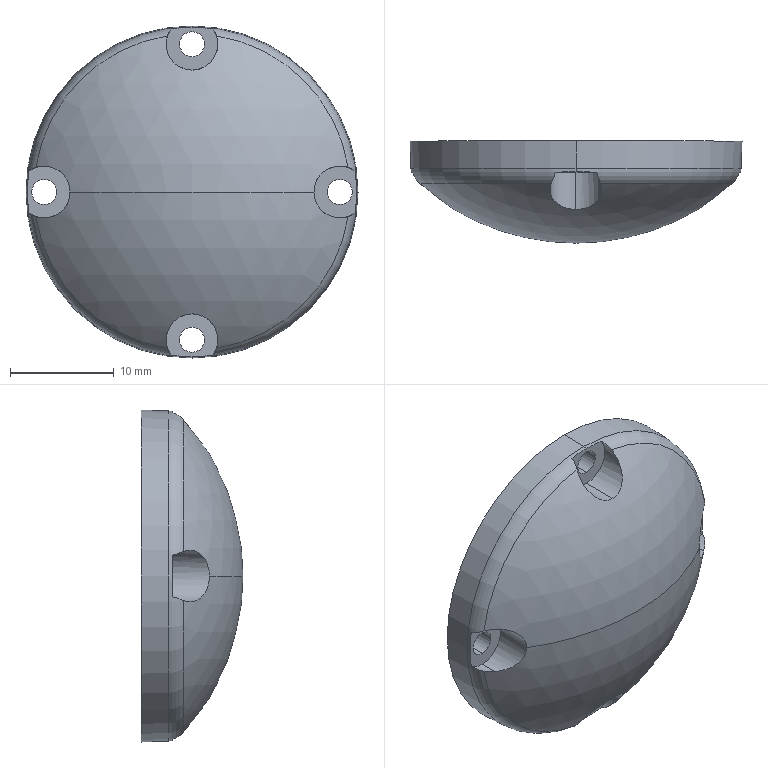Part | SolidWorks | features HoleWzd 1, Revolution 1 | 1 solid | 32 faces | box 32 x 9.828 x 32 mm | volume 4397 mm3 | cylinder 17 | plane 5 | sphere 4 | torus 4 | cone 2 | commonest cylinder face diameters 5 x9 2.4 x8
STEP:
#1=CARTESIAN_POINT('',(-14.25,-5.672,1.2));
#2=VERTEX_POINT('',#1);
#3=CARTESIAN_POINT('',(-14.25,-5.672,-1.2));
#4=VERTEX_POINT('',#3);
#5=CARTESIAN_POINT('',(-14.25,-5.672,0.));
#6=DIRECTION('',(0.,-1.,0.));
#7=DIRECTION('',(0.,0.,-1.));
#8=AXIS2_PLACEMENT_3D('',#5,#6,#7);
#9=CIRCLE('',#8,1.2);
#10=EDGE_CURVE('',#2,#4,#9,.T.);
#11=ORIENTED_EDGE('',*,*,#10,.F.);
#12=CARTESIAN_POINT('',(-14.25,-8.672,1.2));
#13=VERTEX_POINT('',#12);
#14=CARTESIAN_POINT('',(-14.25,-15.672,1.2));
#15=DIRECTION('',(0.,-1.,0.));
#16=VECTOR('',#15,1000.);
#17=LINE('',#14,#16);
#18=EDGE_CURVE('',#2,#13,#17,.T.);
#19=ORIENTED_EDGE('',*,*,#18,.T.);
#20=CARTESIAN_POINT('',(-14.25,-8.672,-1.2));
#21=VERTEX_POINT('',#20);
#22=CARTESIAN_POINT('',(-14.25,-8.672,0.));
#23=DIRECTION('',(0.,-1.,0.));
#24=DIRECTION('',(0.,0.,-1.));
#25=AXIS2_PLACEMENT_3D('',#22,#23,#24);
#26=CIRCLE('',#25,1.2);
#27=EDGE_CURVE('',#13,#21,#26,.T.);
#28=ORIENTED_EDGE('',*,*,#27,.T.);
#29=CARTESIAN_POINT('',(-14.25,-15.672,-1.2));
#30=DIRECTION('',(0.,-1.,0.));
#31=VECTOR('',#30,1000.);
#32=LINE('',#29,#31);
#33=EDGE_CURVE('',#4,#21,#32,.T.);
#34=ORIENTED_EDGE('',*,*,#33,.F.);
#35=EDGE_LOOP('',(#11,#19,#28,#34));
#36=FACE_OUTER_BOUND('',#35,.T.);
#37=CARTESIAN_POINT('',(-14.25,-15.672,0.));
#38=DIRECTION('',(0.,-1.,0.));
#39=DIRECTION('',(0.,0.,-1.));
#40=AXIS2_PLACEMENT_3D('',#37,#38,#39);
#41=CYLINDRICAL_SURFACE('',#40,1.2);
#42=ADVANCED_FACE('',(#36),#41,.F.);
#43=CARTESIAN_POINT('',(-14.25,-8.672,2.5));
#44=VERTEX_POINT('',#43);
#45=CARTESIAN_POINT('',(-15.732,-8.672,2.013));
#46=VERTEX_POINT('',#45);
#47=CARTESIAN_POINT('',(-14.25,-8.672,0.));
#48=DIRECTION('',(0.,-1.,0.));
#49=DIRECTION('',(0.,0.,-1.));
#50=AXIS2_PLACEMENT_3D('',#47,#48,#49);
#51=CIRCLE('',#50,2.5);
#52=EDGE_CURVE('',#44,#46,#51,.T.);
#53=ORIENTED_EDGE('',*,*,#52,.F.);
#54=CARTESIAN_POINT('',(-14.25,-10.38,2.5));
#55=VERTEX_POINT('',#54);
#56=CARTESIAN_POINT('',(-14.25,-15.672,2.5));
#57=DIRECTION('',(0.,-1.,0.));
#58=VECTOR('',#57,1000.);
#59=LINE('',#56,#58);
#60=EDGE_CURVE('',#44,#55,#59,.T.);
#61=ORIENTED_EDGE('',*,*,#60,.T.);
#62=CARTESIAN_POINT('',(-15.049,-9.731,2.369));
#63=VERTEX_POINT('',#62);
#64=CARTESIAN_POINT('',(-15.049,-9.731,2.369));
#65=CARTESIAN_POINT('',(-14.788,-9.947,2.457));
#66=CARTESIAN_POINT('',(-14.522,-10.163,2.5));
#67=CARTESIAN_POINT('',(-14.25,-10.38,2.5));
#68=B_SPLINE_CURVE_WITH_KNOTS('',3,(#64,#65,#66,#67),.UNSPECIFIED.,.F.,.F.,(4,4),(0.00000032,0.001037),.UNSPECIFIED.);
#69=EDGE_CURVE('',#63,#55,#68,.T.);
#70=ORIENTED_EDGE('',*,*,#69,.F.);
#71=CARTESIAN_POINT('',(-15.732,-8.672,2.013));
#72=CARTESIAN_POINT('',(-15.679,-8.886,2.053));
#73=CARTESIAN_POINT('',(-15.591,-9.079,2.114));
#74=CARTESIAN_POINT('',(-15.357,-9.436,2.245));
#75=CARTESIAN_POINT('',(-15.216,-9.594,2.313));
#76=CARTESIAN_POINT('',(-15.049,-9.731,2.369));
#77=B_SPLINE_CURVE_WITH_KNOTS('',3,(#71,#72,#73,#74,#75,#76),.UNSPECIFIED.,.F.,.F.,(4,2,4),(0.000000206,0.0006616,0.001323),.UNSPECIFIED.);
#78=EDGE_CURVE('',#46,#63,#77,.T.);
#79=ORIENTED_EDGE('',*,*,#78,.F.);
#80=EDGE_LOOP('',(#53,#61,#70,#79));
#81=FACE_OUTER_BOUND('',#80,.T.);
#82=CARTESIAN_POINT('',(-14.25,-15.672,0.));
#83=DIRECTION('',(0.,-1.,0.));
#84=DIRECTION('',(0.,0.,-1.));
#85=AXIS2_PLACEMENT_3D('',#82,#83,#84);
#86=CYLINDRICAL_SURFACE('',#85,2.5);
#87=ADVANCED_FACE('',(#81),#86,.F.);
#88=ORIENTED_EDGE('',*,*,#60,.F.);
#89=CARTESIAN_POINT('',(-14.25,-8.672,-2.5));
#90=VERTEX_POINT('',#89);
#91=CARTESIAN_POINT('',(-14.25,-8.672,0.));
#92=DIRECTION('',(0.,-1.,0.));
#93=DIRECTION('',(0.,0.,-1.));
#94=AXIS2_PLACEMENT_3D('',#91,#92,#93);
#95=CIRCLE('',#94,2.5);
#96=EDGE_CURVE('',#90,#44,#95,.T.);
#97=ORIENTED_EDGE('',*,*,#96,.F.);
#98=CARTESIAN_POINT('',(-14.25,-10.38,-2.5));
#99=VERTEX_POINT('',#98);
#100=CARTESIAN_POINT('',(-14.25,-15.672,-2.5));
#101=DIRECTION('',(0.,-1.,0.));
#102=VECTOR('',#101,1000.);
#103=LINE('',#100,#102);
#104=EDGE_CURVE('',#90,#99,#103,.T.);
#105=ORIENTED_EDGE('',*,*,#104,.T.);
#106=CARTESIAN_POINT('',(-11.75,-12.272,0.));
#107=VERTEX_POINT('',#106);
#108=CARTESIAN_POINT('',(-11.75,-12.272,0.));
#109=CARTESIAN_POINT('',(-11.75,-12.272,-0.1848));
#110=CARTESIAN_POINT('',(-11.77,-12.257,-0.3688));
#111=CARTESIAN_POINT('',(-11.851,-12.199,-0.7283));
#112=CARTESIAN_POINT('',(-11.91,-12.156,-0.8982));
#113=CARTESIAN_POINT('',(-12.136,-11.992,-1.381));
#114=CARTESIAN_POINT('',(-12.349,-11.836,-1.655));
#115=CARTESIAN_POINT('',(-12.833,-11.477,-2.085));
#116=CARTESIAN_POINT('',(-13.106,-11.271,-2.243));
#117=CARTESIAN_POINT('',(-13.668,-10.839,-2.45));
#118=CARTESIAN_POINT('',(-13.962,-10.609,-2.5));
#119=CARTESIAN_POINT('',(-14.25,-10.38,-2.5));
#120=B_SPLINE_CURVE_WITH_KNOTS('',3,(#108,#109,#110,#111,#112,#113,#114,#115,#116,#117,#118,#119),.UNSPECIFIED.,.F.,.F.,(4,2,2,2,2,4),(0.005459,0.00601,0.006561,0.007662,0.008764,0.009866),.UNSPECIFIED.);
#121=EDGE_CURVE('',#107,#99,#120,.T.);
#122=ORIENTED_EDGE('',*,*,#121,.F.);
#123=CARTESIAN_POINT('',(-14.25,-10.38,2.5));
#124=CARTESIAN_POINT('',(-14.105,-10.495,2.5));
#125=CARTESIAN_POINT('',(-13.958,-10.611,2.487));
#126=CARTESIAN_POINT('',(-13.671,-10.836,2.436));
#127=CARTESIAN_POINT('',(-13.529,-10.946,2.398));
#128=CARTESIAN_POINT('',(-13.109,-11.268,2.244));
#129=CARTESIAN_POINT('',(-12.834,-11.476,2.086));
#130=CARTESIAN_POINT('',(-12.472,-11.745,1.765));
#131=CARTESIAN_POINT('',(-12.357,-11.83,1.642));
#132=CARTESIAN_POINT('',(-12.152,-11.98,1.371));
#133=CARTESIAN_POINT('',(-12.062,-12.046,1.223));
#134=CARTESIAN_POINT('',(-11.911,-12.156,0.9004));
#135=CARTESIAN_POINT('',(-11.852,-12.199,0.7283));
#136=CARTESIAN_POINT('',(-11.771,-12.257,0.3733));
#137=CARTESIAN_POINT('',(-11.75,-12.272,0.1854));
#138=CARTESIAN_POINT('',(-11.75,-12.272,0.));
#139=B_SPLINE_CURVE_WITH_KNOTS('',3,(#123,#124,#125,#126,#127,#128,#129,#130,#131,#132,#133,#134,#135,#136,#137,#138),.UNSPECIFIED.,.F.,.F.,(4,2,2,2,2,2,2,4),(0.001037,0.00159,0.002142,0.003248,0.003801,0.004353,0.004906,0.005459),.UNSPECIFIED.);
#140=EDGE_CURVE('',#55,#107,#139,.T.);
#141=ORIENTED_EDGE('',*,*,#140,.F.);
#142=EDGE_LOOP('',(#88,#97,#105,#122,#141));
#143=FACE_OUTER_BOUND('',#142,.T.);
#144=CARTESIAN_POINT('',(-14.25,-15.672,0.));
#145=DIRECTION('',(0.,-1.,0.));
#146=DIRECTION('',(0.,0.,-1.));
#147=AXIS2_PLACEMENT_3D('',#144,#145,#146);
#148=CYLINDRICAL_SURFACE('',#147,2.5);
#149=ADVANCED_FACE('',(#143),#148,.F.);
#150=CARTESIAN_POINT('',(0.,-5.672,-13.05));
#151=VERTEX_POINT('',#150);
#152=CARTESIAN_POINT('',(0.,-5.672,-15.45));
#153=VERTEX_POINT('',#152);
#154=CARTESIAN_POINT('',(0.,-5.672,-14.25));
#155=DIRECTION('',(0.,-1.,0.));
#156=DIRECTION('',(0.,0.,-1.));
#157=AXIS2_PLACEMENT_3D('',#154,#155,#156);
#158=CIRCLE('',#157,1.2);
#159=EDGE_CURVE('',#151,#153,#158,.T.);
#160=ORIENTED_EDGE('',*,*,#159,.F.);
#161=CARTESIAN_POINT('',(0.,-8.672,-13.05));
#162=VERTEX_POINT('',#161);
#163=CARTESIAN_POINT('',(0.,-15.672,-13.05));
#164=DIRECTION('',(0.,-1.,0.));
#165=VECTOR('',#164,1000.);
#166=LINE('',#163,#165);
#167=EDGE_CURVE('',#151,#162,#166,.T.);
#168=ORIENTED_EDGE('',*,*,#167,.T.);
#169=CARTESIAN_POINT('',(0.,-8.672,-15.45));
#170=VERTEX_POINT('',#169);
#171=CARTESIAN_POINT('',(0.,-8.672,-14.25));
#172=DIRECTION('',(0.,-1.,0.));
#173=DIRECTION('',(0.,0.,-1.));
#174=AXIS2_PLACEMENT_3D('',#171,#172,#173);
#175=CIRCLE('',#174,1.2);
#176=EDGE_CURVE('',#162,#170,#175,.T.);
#177=ORIENTED_EDGE('',*,*,#176,.T.);
#178=CARTESIAN_POINT('',(0.,-15.672,-15.45));
#179=DIRECTION('',(0.,-1.,0.));
#180=VECTOR('',#179,1000.);
#181=LINE('',#178,#180);
#182=EDGE_CURVE('',#153,#170,#181,.T.);
#183=ORIENTED_EDGE('',*,*,#182,.F.);
#184=EDGE_LOOP('',(#160,#168,#177,#183));
#185=FACE_OUTER_BOUND('',#184,.T.);
#186=CARTESIAN_POINT('',(0.,-15.672,-14.25));
#187=DIRECTION('',(0.,-1.,0.));
#188=DIRECTION('',(0.,0.,-1.));
#189=AXIS2_PLACEMENT_3D('',#186,#187,#188);
#190=CYLINDRICAL_SURFACE('',#189,1.2);
#191=ADVANCED_FACE('',(#185),#190,.F.);
#192=CARTESIAN_POINT('',(14.25,-5.672,1.2));
#193=VERTEX_POINT('',#192);
#194=CARTESIAN_POINT('',(14.25,-5.672,-1.2));
#195=VERTEX_POINT('',#194);
#196=CARTESIAN_POINT('',(14.25,-5.672,0.));
#197=DIRECTION('',(0.,-1.,0.));
#198=DIRECTION('',(0.,0.,-1.));
#199=AXIS2_PLACEMENT_3D('',#196,#197,#198);
#200=CIRCLE('',#199,1.2);
#201=EDGE_CURVE('',#193,#195,#200,.T.);
#202=ORIENTED_EDGE('',*,*,#201,.F.);
#203=CARTESIAN_POINT('',(14.25,-8.672,1.2));
#204=VERTEX_POINT('',#203);
#205=CARTESIAN_POINT('',(14.25,-15.672,1.2));
#206=DIRECTION('',(0.,-1.,0.));
#207=VECTOR('',#206,1000.);
#208=LINE('',#205,#207);
#209=EDGE_CURVE('',#193,#204,#208,.T.);
#210=ORIENTED_EDGE('',*,*,#209,.T.);
#211=CARTESIAN_POINT('',(14.25,-8.672,-1.2));
#212=VERTEX_POINT('',#211);
#213=CARTESIAN_POINT('',(14.25,-8.672,0.));
#214=DIRECTION('',(0.,-1.,0.));
#215=DIRECTION('',(0.,0.,-1.));
#216=AXIS2_PLACEMENT_3D('',#213,#214,#215);
#217=CIRCLE('',#216,1.2);
#218=EDGE_CURVE('',#204,#212,#217,.T.);
#219=ORIENTED_EDGE('',*,*,#218,.T.);
#220=CARTESIAN_POINT('',(14.25,-15.672,-1.2));
#221=DIRECTION('',(0.,-1.,0.));
#222=VECTOR('',#221,1000.);
#223=LINE('',#220,#222);
#224=EDGE_CURVE('',#195,#212,#223,.T.);
#225=ORIENTED_EDGE('',*,*,#224,.F.);
#226=EDGE_LOOP('',(#202,#210,#219,#225));
#227=FACE_OUTER_BOUND('',#226,.T.);
#228=CARTESIAN_POINT('',(14.25,-15.672,0.));
#229=DIRECTION('',(0.,-1.,0.));
#230=DIRECTION('',(0.,0.,-1.));
#231=AXIS2_PLACEMENT_3D('',#228,#229,#230);
#232=CYLINDRICAL_SURFACE('',#231,1.2);
#233=ADVANCED_FACE('',(#227),#232,.F.);
#234=CARTESIAN_POINT('',(14.25,-8.672,2.5));
#235=VERTEX_POINT('',#234);
#236=CARTESIAN_POINT('',(14.25,-8.672,-2.5));
#237=VERTEX_POINT('',#236);
#238=CARTESIAN_POINT('',(14.25,-8.672,0.));
#239=DIRECTION('',(0.,-1.,0.));
#240=DIRECTION('',(0.,0.,-1.));
#241=AXIS2_PLACEMENT_3D('',#238,#239,#240);
#242=CIRCLE('',#241,2.5);
#243=EDGE_CURVE('',#235,#237,#242,.T.);
#244=ORIENTED_EDGE('',*,*,#243,.F.);
#245=CARTESIAN_POINT('',(14.25,-10.38,2.5));
#246=VERTEX_POINT('',#245);
#247=CARTESIAN_POINT('',(14.25,-15.672,2.5));
#248=DIRECTION('',(0.,-1.,0.));
#249=VECTOR('',#248,1000.);
#250=LINE('',#247,#249);
#251=EDGE_CURVE('',#235,#246,#250,.T.);
#252=ORIENTED_EDGE('',*,*,#251,.T.);
#253=CARTESIAN_POINT('',(11.75,-12.272,0.));
#254=VERTEX_POINT('',#253);
#255=CARTESIAN_POINT('',(11.75,-12.272,0.));
#256=CARTESIAN_POINT('',(11.75,-12.272,0.1848));
#257=CARTESIAN_POINT('',(11.77,-12.257,0.3688));
#258=CARTESIAN_POINT('',(11.851,-12.199,0.7283));
#259=CARTESIAN_POINT('',(11.91,-12.156,0.8982));
#260=CARTESIAN_POINT('',(12.136,-11.992,1.381));
#261=CARTESIAN_POINT('',(12.349,-11.836,1.655));
#262=CARTESIAN_POINT('',(12.833,-11.477,2.085));
#263=CARTESIAN_POINT('',(13.106,-11.271,2.243));
#264=CARTESIAN_POINT('',(13.668,-10.839,2.45));
#265=CARTESIAN_POINT('',(13.962,-10.609,2.5));
#266=CARTESIAN_POINT('',(14.25,-10.38,2.5));
#267=B_SPLINE_CURVE_WITH_KNOTS('',3,(#255,#256,#257,#258,#259,#260,#261,#262,#263,#264,#265,#266),.UNSPECIFIED.,.F.,.F.,(4,2,2,2,2,4),(0.005459,0.00601,0.006561,0.007662,0.008764,0.009866),.UNSPECIFIED.);
#268=EDGE_CURVE('',#254,#246,#267,.T.);
#269=ORIENTED_EDGE('',*,*,#268,.F.);
#270=CARTESIAN_POINT('',(14.25,-10.38,-2.5));
#271=VERTEX_POINT('',#270);
#272=CARTESIAN_POINT('',(14.25,-10.38,-2.5));
#273=CARTESIAN_POINT('',(14.105,-10.495,-2.5));
#274=CARTESIAN_POINT('',(13.958,-10.611,-2.487));
#275=CARTESIAN_POINT('',(13.671,-10.836,-2.436));
#276=CARTESIAN_POINT('',(13.529,-10.946,-2.398));
#277=CARTESIAN_POINT('',(13.109,-11.268,-2.244));
#278=CARTESIAN_POINT('',(12.834,-11.476,-2.086));
#279=CARTESIAN_POINT('',(12.472,-11.745,-1.765));
#280=CARTESIAN_POINT('',(12.357,-11.83,-1.642));
#281=CARTESIAN_POINT('',(12.152,-11.98,-1.371));
#282=CARTESIAN_POINT('',(12.062,-12.046,-1.223));
#283=CARTESIAN_POINT('',(11.911,-12.156,-0.9004));
#284=CARTESIAN_POINT('',(11.852,-12.199,-0.7283));
#285=CARTESIAN_POINT('',(11.771,-12.257,-0.3733));
#286=CARTESIAN_POINT('',(11.75,-12.272,-0.1854));
#287=CARTESIAN_POINT('',(11.75,-12.272,0.));
#288=B_SPLINE_CURVE_WITH_KNOTS('',3,(#272,#273,#274,#275,#276,#277,#278,#279,#280,#281,#282,#283,#284,#285,#286,#287),.UNSPECIFIED.,.F.,.F.,(4,2,2,2,2,2,2,4),(0.001037,0.00159,0.002142,0.003248,0.003801,0.004353,0.004906,0.005459),.UNSPECIFIED.);
#289=EDGE_CURVE('',#271,#254,#288,.T.);
#290=ORIENTED_EDGE('',*,*,#289,.F.);
#291=CARTESIAN_POINT('',(14.25,-15.672,-2.5));
#292=DIRECTION('',(0.,-1.,0.));
#293=VECTOR('',#292,1000.);
#294=LINE('',#291,#293);
#295=EDGE_CURVE('',#237,#271,#294,.T.);
#296=ORIENTED_EDGE('',*,*,#295,.F.);
#297=EDGE_LOOP('',(#244,#252,#269,#290,#296));
#298=FACE_OUTER_BOUND('',#297,.T.);
#299=CARTESIAN_POINT('',(14.25,-15.672,0.));
#300=DIRECTION('',(0.,-1.,0.));
#301=DIRECTION('',(0.,0.,-1.));
#302=AXIS2_PLACEMENT_3D('',#299,#300,#301);
#303=CYLINDRICAL_SURFACE('',#302,2.5);
#304=ADVANCED_FACE('',(#298),#303,.F.);
#305=CARTESIAN_POINT('',(15.732,-8.672,-2.013));
#306=VERTEX_POINT('',#305);
#307=CARTESIAN_POINT('',(14.25,-8.672,0.));
#308=DIRECTION('',(0.,-1.,0.));
#309=DIRECTION('',(0.,0.,-1.));
#310=AXIS2_PLACEMENT_3D('',#307,#308,#309);
#311=CIRCLE('',#310,2.5);
#312=EDGE_CURVE('',#237,#306,#311,.T.);
#313=ORIENTED_EDGE('',*,*,#312,.F.);
#314=ORIENTED_EDGE('',*,*,#295,.T.);
#315=CARTESIAN_POINT('',(15.049,-9.731,-2.369));
#316=VERTEX_POINT('',#315);
#317=CARTESIAN_POINT('',(15.049,-9.731,-2.369));
#318=CARTESIAN_POINT('',(14.788,-9.947,-2.457));
#319=CARTESIAN_POINT('',(14.522,-10.163,-2.5));
#320=CARTESIAN_POINT('',(14.25,-10.38,-2.5));
#321=B_SPLINE_CURVE_WITH_KNOTS('',3,(#317,#318,#319,#320),.UNSPECIFIED.,.F.,.F.,(4,4),(0.00000032,0.001037),.UNSPECIFIED.);
#322=EDGE_CURVE('',#316,#271,#321,.T.);
#323=ORIENTED_EDGE('',*,*,#322,.F.);
#324=CARTESIAN_POINT('',(15.732,-8.672,-2.013));
#325=CARTESIAN_POINT('',(15.679,-8.886,-2.053));
#326=CARTESIAN_POINT('',(15.591,-9.079,-2.114));
#327=CARTESIAN_POINT('',(15.357,-9.436,-2.245));
#328=CARTESIAN_POINT('',(15.216,-9.594,-2.313));
#329=CARTESIAN_POINT('',(15.049,-9.731,-2.369));
#330=B_SPLINE_CURVE_WITH_KNOTS('',3,(#324,#325,#326,#327,#328,#329),.UNSPECIFIED.,.F.,.F.,(4,2,4),(0.000000206,0.0006616,0.001323),.UNSPECIFIED.);
#331=EDGE_CURVE('',#306,#316,#330,.T.);
#332=ORIENTED_EDGE('',*,*,#331,.F.);
#333=EDGE_LOOP('',(#313,#314,#323,#332));
#334=FACE_OUTER_BOUND('',#333,.T.);
#335=CARTESIAN_POINT('',(14.25,-15.672,0.));
#336=DIRECTION('',(0.,-1.,0.));
#337=DIRECTION('',(0.,0.,-1.));
#338=AXIS2_PLACEMENT_3D('',#335,#336,#337);
#339=CYLINDRICAL_SURFACE('',#338,2.5);
#340=ADVANCED_FACE('',(#334),#339,.F.);
#341=CARTESIAN_POINT('',(0.,-5.672,15.45));
#342=VERTEX_POINT('',#341);
#343=CARTESIAN_POINT('',(0.,-5.672,13.05));
#344=VERTEX_POINT('',#343);
#345=CARTESIAN_POINT('',(0.,-5.672,14.25));
#346=DIRECTION('',(0.,-1.,0.));
#347=DIRECTION('',(0.,0.,-1.));
#348=AXIS2_PLACEMENT_3D('',#345,#346,#347);
#349=CIRCLE('',#348,1.2);
#350=EDGE_CURVE('',#342,#344,#349,.T.);
#351=ORIENTED_EDGE('',*,*,#350,.F.);
#352=CARTESIAN_POINT('',(0.,-8.672,15.45));
#353=VERTEX_POINT('',#352);
#354=CARTESIAN_POINT('',(0.,-15.672,15.45));
#355=DIRECTION('',(0.,-1.,0.));
#356=VECTOR('',#355,1000.);
#357=LINE('',#354,#356);
#358=EDGE_CURVE('',#342,#353,#357,.T.);
#359=ORIENTED_EDGE('',*,*,#358,.T.);
#360=CARTESIAN_POINT('',(0.,-8.672,13.05));
#361=VERTEX_POINT('',#360);
#362=CARTESIAN_POINT('',(0.,-8.672,14.25));
#363=DIRECTION('',(0.,-1.,0.));
#364=DIRECTION('',(0.,0.,-1.));
#365=AXIS2_PLACEMENT_3D('',#362,#363,#364);
#366=CIRCLE('',#365,1.2);
#367=EDGE_CURVE('',#353,#361,#366,.T.);
#368=ORIENTED_EDGE('',*,*,#367,.T.);
#369=CARTESIAN_POINT('',(0.,-15.672,13.05));
#370=DIRECTION('',(0.,-1.,0.));
#371=VECTOR('',#370,1000.);
#372=LINE('',#369,#371);
#373=EDGE_CURVE('',#344,#361,#372,.T.);
#374=ORIENTED_EDGE('',*,*,#373,.F.);
#375=EDGE_LOOP('',(#351,#359,#368,#374));
#376=FACE_OUTER_BOUND('',#375,.T.);
#377=CARTESIAN_POINT('',(0.,-15.672,14.25));
#378=DIRECTION('',(0.,-1.,0.));
#379=DIRECTION('',(0.,0.,-1.));
#380=AXIS2_PLACEMENT_3D('',#377,#378,#379);
#381=CYLINDRICAL_SURFACE('',#380,1.2);
#382=ADVANCED_FACE('',(#376),#381,.F.);
#383=CARTESIAN_POINT('',(0.,-8.672,11.75));
#384=VERTEX_POINT('',#383);
#385=CARTESIAN_POINT('',(2.013,-8.672,15.732));
#386=VERTEX_POINT('',#385);
#387=CARTESIAN_POINT('',(0.,-8.672,14.25));
#388=DIRECTION('',(0.,-1.,0.));
#389=DIRECTION('',(0.,0.,-1.));
#390=AXIS2_PLACEMENT_3D('',#387,#388,#389);
#391=CIRCLE('',#390,2.5);
#392=EDGE_CURVE('',#384,#386,#391,.T.);
#393=ORIENTED_EDGE('',*,*,#392,.F.);
#394=CARTESIAN_POINT('',(0.,-12.272,11.75));
#395=VERTEX_POINT('',#394);
#396=CARTESIAN_POINT('',(0.,-15.672,11.75));
#397=DIRECTION('',(0.,-1.,0.));
#398=VECTOR('',#397,1000.);
#399=LINE('',#396,#398);
#400=EDGE_CURVE('',#384,#395,#399,.T.);
#401=ORIENTED_EDGE('',*,*,#400,.T.);
#402=CARTESIAN_POINT('',(2.369,-9.731,15.049));
#403=VERTEX_POINT('',#402);
#404=CARTESIAN_POINT('',(2.369,-9.731,15.049));
#405=CARTESIAN_POINT('',(2.427,-9.873,14.877));
#406=CARTESIAN_POINT('',(2.465,-10.016,14.703));
#407=CARTESIAN_POINT('',(2.504,-10.3,14.35));
#408=CARTESIAN_POINT('',(2.505,-10.444,14.17));
#409=CARTESIAN_POINT('',(2.468,-10.727,13.811));
#410=CARTESIAN_POINT('',(2.43,-10.864,13.635));
#411=CARTESIAN_POINT('',(2.315,-11.132,13.288));
#412=CARTESIAN_POINT('',(2.236,-11.262,13.116));
#413=CARTESIAN_POINT('',(2.036,-11.511,12.786));
#414=CARTESIAN_POINT('',(1.915,-11.627,12.631));
#415=CARTESIAN_POINT('',(1.63,-11.84,12.343));
#416=CARTESIAN_POINT('',(1.463,-11.937,12.212));
#417=CARTESIAN_POINT('',(1.096,-12.096,11.993));
#418=CARTESIAN_POINT('',(0.8895,-12.162,11.903));
#419=CARTESIAN_POINT('',(0.5669,-12.227,11.813));
#420=CARTESIAN_POINT('',(0.4568,-12.244,11.789));
#421=CARTESIAN_POINT('',(0.2308,-12.266,11.758));
#422=CARTESIAN_POINT('',(0.1145,-12.272,11.75));
#423=CARTESIAN_POINT('',(0.,-12.272,11.75));
#424=B_SPLINE_CURVE_WITH_KNOTS('',3,(#404,#405,#406,#407,#408,#409,#410,#411,#412,#413,#414,#415,#416,#417,#418,#419,#420,#421,#422,#423),.UNSPECIFIED.,.F.,.F.,(4,2,2,2,2,2,2,2,2,4),(0.00000032,0.0006827,0.001365,0.002047,0.00273,0.003412,0.004094,0.004777,0.005118,0.005459),.UNSPECIFIED.);
#425=EDGE_CURVE('',#403,#395,#424,.T.);
#426=ORIENTED_EDGE('',*,*,#425,.F.);
#427=CARTESIAN_POINT('',(2.013,-8.672,15.732));
#428=CARTESIAN_POINT('',(2.053,-8.886,15.679));
#429=CARTESIAN_POINT('',(2.114,-9.079,15.591));
#430=CARTESIAN_POINT('',(2.245,-9.436,15.357));
#431=CARTESIAN_POINT('',(2.313,-9.594,15.216));
#432=CARTESIAN_POINT('',(2.369,-9.731,15.049));
#433=B_SPLINE_CURVE_WITH_KNOTS('',3,(#427,#428,#429,#430,#431,#432),.UNSPECIFIED.,.F.,.F.,(4,2,4),(0.000000206,0.0006616,0.001323),.UNSPECIFIED.);
#434=EDGE_CURVE('',#386,#403,#433,.T.);
#435=ORIENTED_EDGE('',*,*,#434,.F.);
#436=EDGE_LOOP('',(#393,#401,#426,#435));
#437=FACE_OUTER_BOUND('',#436,.T.);
#438=CARTESIAN_POINT('',(0.,-15.672,14.25));
#439=DIRECTION('',(0.,-1.,0.));
#440=DIRECTION('',(0.,0.,-1.));
#441=AXIS2_PLACEMENT_3D('',#438,#439,#440);
#442=CYLINDRICAL_SURFACE('',#441,2.5);
#443=ADVANCED_FACE('',(#437),#442,.F.);
#444=CARTESIAN_POINT('',(0.,-11.,0.));
#445=VERTEX_POINT('',#444);
#446=CARTESIAN_POINT('',(9.143,-6.116,0.));
#447=VERTEX_POINT('',#446);
#448=CARTESIAN_POINT('',(0.,0.,0.));
#449=DIRECTION('',(0.,0.,1.));
#450=DIRECTION('',(1.,0.,0.));
#451=AXIS2_PLACEMENT_3D('',#448,#449,#450);
#452=CIRCLE('',#451,11.);
#453=EDGE_CURVE('',#445,#447,#452,.T.);
#454=ORIENTED_EDGE('',*,*,#453,.F.);
#455=CARTESIAN_POINT('',(-9.143,-6.116,0.));
#456=VERTEX_POINT('',#455);
#457=CARTESIAN_POINT('',(0.,0.,0.));
#458=DIRECTION('',(0.,0.,-1.));
#459=DIRECTION('',(-1.,0.,0.));
#460=AXIS2_PLACEMENT_3D('',#457,#458,#459);
#461=CIRCLE('',#460,11.);
#462=EDGE_CURVE('',#445,#456,#461,.T.);
#463=ORIENTED_EDGE('',*,*,#462,.T.);
#464=CARTESIAN_POINT('',(0.,-6.116,9.143));
#465=VERTEX_POINT('',#464);
#466=CARTESIAN_POINT('',(0.,-6.116,0.));
#467=DIRECTION('',(0.,1.,0.));
#468=DIRECTION('',(0.,0.,1.));
#469=AXIS2_PLACEMENT_3D('',#466,#467,#468);
#470=CIRCLE('',#469,9.143);
#471=EDGE_CURVE('',#456,#465,#470,.T.);
#472=ORIENTED_EDGE('',*,*,#471,.T.);
#473=CARTESIAN_POINT('',(0.,-6.116,0.));
#474=DIRECTION('',(0.,1.,0.));
#475=DIRECTION('',(0.,0.,1.));
#476=AXIS2_PLACEMENT_3D('',#473,#474,#475);
#477=CIRCLE('',#476,9.143);
#478=EDGE_CURVE('',#465,#447,#477,.T.);
#479=ORIENTED_EDGE('',*,*,#478,.T.);
#480=EDGE_LOOP('',(#454,#463,#472,#479));
#481=FACE_OUTER_BOUND('',#480,.T.);
#482=CARTESIAN_POINT('',(0.,0.,0.));
#483=DIRECTION('',(0.,0.,-1.));
#484=DIRECTION('',(1.,0.,0.));
#485=AXIS2_PLACEMENT_3D('',#482,#483,#484);
#486=SPHERICAL_SURFACE('',#485,11.);
#487=ADVANCED_FACE('',(#481),#486,.F.);
#488=CARTESIAN_POINT('',(0.,-5.672,9.974));
#489=VERTEX_POINT('',#488);
#490=CARTESIAN_POINT('',(0.,-5.672,-9.974));
#491=VERTEX_POINT('',#490);
#492=CARTESIAN_POINT('',(0.,-5.672,0.));
#493=DIRECTION('',(0.,1.,0.));
#494=DIRECTION('',(0.,0.,1.));
#495=AXIS2_PLACEMENT_3D('',#492,#493,#494);
#496=CIRCLE('',#495,9.974);
#497=EDGE_CURVE('',#489,#491,#496,.T.);
#498=ORIENTED_EDGE('',*,*,#497,.T.);
#499=CARTESIAN_POINT('',(0.,-6.116,-9.143));
#500=VERTEX_POINT('',#499);
#501=CARTESIAN_POINT('',(0.,-6.672,-9.974));
#502=DIRECTION('',(1.,0.,0.));
#503=DIRECTION('',(0.,0.,-1.));
#504=AXIS2_PLACEMENT_3D('',#501,#502,#503);
#505=CIRCLE('',#504,1.);
#506=EDGE_CURVE('',#491,#500,#505,.T.);
#507=ORIENTED_EDGE('',*,*,#506,.T.);
#508=CARTESIAN_POINT('',(0.,-6.116,0.));
#509=DIRECTION('',(0.,1.,0.));
#510=DIRECTION('',(0.,0.,1.));
#511=AXIS2_PLACEMENT_3D('',#508,#509,#510);
#512=CIRCLE('',#511,9.143);
#513=EDGE_CURVE('',#447,#500,#512,.T.);
#514=ORIENTED_EDGE('',*,*,#513,.F.);
#515=ORIENTED_EDGE('',*,*,#478,.F.);
#516=CARTESIAN_POINT('',(0.,-6.672,9.974));
#517=DIRECTION('',(-1.,0.,0.));
#518=DIRECTION('',(0.,0.,1.));
#519=AXIS2_PLACEMENT_3D('',#516,#517,#518);
#520=CIRCLE('',#519,1.);
#521=EDGE_CURVE('',#489,#465,#520,.T.);
#522=ORIENTED_EDGE('',*,*,#521,.F.);
#523=EDGE_LOOP('',(#498,#507,#514,#515,#522));
#524=FACE_OUTER_BOUND('',#523,.T.);
#525=CARTESIAN_POINT('',(0.,-6.672,0.));
#526=DIRECTION('',(0.,1.,0.));
#527=DIRECTION('',(0.,0.,1.));
#528=AXIS2_PLACEMENT_3D('',#525,#526,#527);
#529=TOROIDAL_SURFACE('',#528,9.974,1.);
#530=ADVANCED_FACE('',(#524),#529,.T.);
#531=CARTESIAN_POINT('',(0.,-8.303,15.908));
#532=VERTEX_POINT('',#531);
#533=CARTESIAN_POINT('',(0.,-8.303,-15.908));
#534=VERTEX_POINT('',#533);
#535=CARTESIAN_POINT('',(0.,-8.303,0.));
#536=DIRECTION('',(0.,1.,0.));
#537=DIRECTION('',(0.,0.,1.));
#538=AXIS2_PLACEMENT_3D('',#535,#536,#537);
#539=CIRCLE('',#538,15.908);
#540=EDGE_CURVE('',#532,#534,#539,.T.);
#541=ORIENTED_EDGE('',*,*,#540,.T.);
#542=CARTESIAN_POINT('',(0.,-5.672,-16.));
#543=VERTEX_POINT('',#542);
#544=CARTESIAN_POINT('',(0.,-8.303,-15.908));
#545=DIRECTION('',(0.,0.9994,-0.0349));
#546=VECTOR('',#545,1000.);
#547=LINE('',#544,#546);
#548=EDGE_CURVE('',#534,#543,#547,.T.);
#549=ORIENTED_EDGE('',*,*,#548,.T.);
#550=CARTESIAN_POINT('',(0.,-5.672,16.));
#551=VERTEX_POINT('',#550);
#552=CARTESIAN_POINT('',(0.,-5.672,0.));
#553=DIRECTION('',(0.,1.,0.));
#554=DIRECTION('',(0.,0.,1.));
#555=AXIS2_PLACEMENT_3D('',#552,#553,#554);
#556=CIRCLE('',#555,16.);
#557=EDGE_CURVE('',#551,#543,#556,.T.);
#558=ORIENTED_EDGE('',*,*,#557,.F.);
#559=CARTESIAN_POINT('',(0.,-8.303,15.908));
#560=DIRECTION('',(0.,0.9994,0.0349));
#561=VECTOR('',#560,1000.);
#562=LINE('',#559,#561);
#563=EDGE_CURVE('',#532,#551,#562,.T.);
#564=ORIENTED_EDGE('',*,*,#563,.F.);
#565=EDGE_LOOP('',(#541,#549,#558,#564));
#566=FACE_OUTER_BOUND('',#565,.T.);
#567=CARTESIAN_POINT('',(0.,-8.303,0.));
#568=DIRECTION('',(0.,1.,0.));
#569=DIRECTION('',(0.,0.,1.));
#570=AXIS2_PLACEMENT_3D('',#567,#568,#569);
#571=CONICAL_SURFACE('',#570,15.908,0.03491);
#572=ADVANCED_FACE('',(#566),#571,.T.);
#573=CARTESIAN_POINT('',(2.013,-8.672,-15.732));
#574=VERTEX_POINT('',#573);
#575=CARTESIAN_POINT('',(0.,-8.672,-15.861));
#576=VERTEX_POINT('',#575);
#577=CARTESIAN_POINT('',(0.,-8.672,0.));
#578=DIRECTION('',(0.,1.,0.));
#579=DIRECTION('',(0.,0.,1.));
#580=AXIS2_PLACEMENT_3D('',#577,#578,#579);
#581=CIRCLE('',#580,15.861);
#582=EDGE_CURVE('',#574,#576,#581,.T.);
#583=ORIENTED_EDGE('',*,*,#582,.T.);
#584=CARTESIAN_POINT('',(0.,-8.233,-13.909));
#585=DIRECTION('',(1.,0.,0.));
#586=DIRECTION('',(0.,0.,-1.));
#587=AXIS2_PLACEMENT_3D('',#584,#585,#586);
#588=CIRCLE('',#587,2.);
#589=EDGE_CURVE('',#576,#534,#588,.T.);
#590=ORIENTED_EDGE('',*,*,#589,.T.);
#591=ORIENTED_EDGE('',*,*,#540,.F.);
#592=CARTESIAN_POINT('',(0.,-8.672,15.861));
#593=VERTEX_POINT('',#592);
#594=CARTESIAN_POINT('',(0.,-8.233,13.909));
#595=DIRECTION('',(-1.,0.,0.));
#596=DIRECTION('',(0.,0.,1.));
#597=AXIS2_PLACEMENT_3D('',#594,#595,#596);
#598=CIRCLE('',#597,2.);
#599=EDGE_CURVE('',#593,#532,#598,.T.);
#600=ORIENTED_EDGE('',*,*,#599,.F.);
#601=CARTESIAN_POINT('',(0.,-8.672,0.));
#602=DIRECTION('',(0.,1.,0.));
#603=DIRECTION('',(0.,0.,1.));
#604=AXIS2_PLACEMENT_3D('',#601,#602,#603);
#605=CIRCLE('',#604,15.861);
#606=EDGE_CURVE('',#593,#386,#605,.T.);
#607=ORIENTED_EDGE('',*,*,#606,.T.);
#608=ORIENTED_EDGE('',*,*,#434,.T.);
#609=CARTESIAN_POINT('',(15.049,-9.731,2.369));
#610=VERTEX_POINT('',#609);
#611=CARTESIAN_POINT('',(0.,-9.731,0.));
#612=DIRECTION('',(0.,1.,0.));
#613=DIRECTION('',(0.,0.,1.));
#614=AXIS2_PLACEMENT_3D('',#611,#612,#613);
#615=CIRCLE('',#614,15.234);
#616=EDGE_CURVE('',#403,#610,#615,.T.);
#617=ORIENTED_EDGE('',*,*,#616,.T.);
#618=CARTESIAN_POINT('',(15.732,-8.672,2.013));
#619=VERTEX_POINT('',#618);
#620=CARTESIAN_POINT('',(15.049,-9.731,2.369));
#621=CARTESIAN_POINT('',(15.216,-9.593,2.313));
#622=CARTESIAN_POINT('',(15.356,-9.437,2.246));
#623=CARTESIAN_POINT('',(15.59,-9.081,2.115));
#624=CARTESIAN_POINT('',(15.679,-8.886,2.053));
#625=CARTESIAN_POINT('',(15.732,-8.672,2.013));
#626=B_SPLINE_CURVE_WITH_KNOTS('',3,(#620,#621,#622,#623,#624,#625),.UNSPECIFIED.,.F.,.F.,(4,2,4),(0.00000032,0.0006625,0.001325),.UNSPECIFIED.);
#627=EDGE_CURVE('',#610,#619,#626,.T.);
#628=ORIENTED_EDGE('',*,*,#627,.T.);
#629=CARTESIAN_POINT('',(0.,-8.672,0.));
#630=DIRECTION('',(0.,1.,0.));
#631=DIRECTION('',(0.,0.,1.));
#632=AXIS2_PLACEMENT_3D('',#629,#630,#631);
#633=CIRCLE('',#632,15.861);
#634=EDGE_CURVE('',#619,#306,#633,.T.);
#635=ORIENTED_EDGE('',*,*,#634,.T.);
#636=ORIENTED_EDGE('',*,*,#331,.T.);
#637=CARTESIAN_POINT('',(2.369,-9.731,-15.049));
#638=VERTEX_POINT('',#637);
#639=CARTESIAN_POINT('',(0.,-9.731,0.));
#640=DIRECTION('',(0.,1.,0.));
#641=DIRECTION('',(0.,0.,1.));
#642=AXIS2_PLACEMENT_3D('',#639,#640,#641);
#643=CIRCLE('',#642,15.234);
#644=EDGE_CURVE('',#316,#638,#643,.T.);
#645=ORIENTED_EDGE('',*,*,#644,.T.);
#646=CARTESIAN_POINT('',(2.369,-9.731,-15.049));
#647=CARTESIAN_POINT('',(2.313,-9.593,-15.216));
#648=CARTESIAN_POINT('',(2.246,-9.437,-15.356));
#649=CARTESIAN_POINT('',(2.115,-9.081,-15.59));
#650=CARTESIAN_POINT('',(2.053,-8.886,-15.679));
#651=CARTESIAN_POINT('',(2.013,-8.672,-15.732));
#652=B_SPLINE_CURVE_WITH_KNOTS('',3,(#646,#647,#648,#649,#650,#651),.UNSPECIFIED.,.F.,.F.,(4,2,4),(0.00000032,0.0006625,0.001325),.UNSPECIFIED.);
#653=EDGE_CURVE('',#638,#574,#652,.T.);
#654=ORIENTED_EDGE('',*,*,#653,.T.);
#655=EDGE_LOOP('',(#583,#590,#591,#600,#607,#608,#617,#628,#635,#636,#645,#654));
#656=FACE_OUTER_BOUND('',#655,.T.);
#657=CARTESIAN_POINT('',(0.,-8.233,0.));
#658=DIRECTION('',(0.,1.,0.));
#659=DIRECTION('',(0.,0.,1.));
#660=AXIS2_PLACEMENT_3D('',#657,#658,#659);
#661=TOROIDAL_SURFACE('',#660,13.909,2.);
#662=ADVANCED_FACE('',(#656),#661,.T.);
#663=CARTESIAN_POINT('',(0.,-15.5,0.));
#664=VERTEX_POINT('',#663);
#665=CARTESIAN_POINT('',(0.,7.5,0.));
#666=DIRECTION('',(0.,0.,1.));
#667=DIRECTION('',(1.,0.,0.));
#668=AXIS2_PLACEMENT_3D('',#665,#666,#667);
#669=CIRCLE('',#668,23.);
#670=EDGE_CURVE('',#664,#254,#669,.T.);
#671=ORIENTED_EDGE('',*,*,#670,.F.);
#672=CARTESIAN_POINT('',(0.,7.5,0.));
#673=DIRECTION('',(0.,0.,-1.));
#674=DIRECTION('',(-1.,0.,0.));
#675=AXIS2_PLACEMENT_3D('',#672,#673,#674);
#676=CIRCLE('',#675,23.);
#677=EDGE_CURVE('',#664,#107,#676,.T.);
#678=ORIENTED_EDGE('',*,*,#677,.T.);
#679=ORIENTED_EDGE('',*,*,#121,.T.);
#680=CARTESIAN_POINT('',(-15.049,-9.731,-2.369));
#681=VERTEX_POINT('',#680);
#682=CARTESIAN_POINT('',(-14.25,-10.38,-2.5));
#683=CARTESIAN_POINT('',(-14.519,-10.165,-2.5));
#684=CARTESIAN_POINT('',(-14.789,-9.946,-2.457));
#685=CARTESIAN_POINT('',(-15.049,-9.731,-2.369));
#686=B_SPLINE_CURVE_WITH_KNOTS('',3,(#682,#683,#684,#685),.UNSPECIFIED.,.F.,.F.,(4,4),(0.009866,0.0109),.UNSPECIFIED.);
#687=EDGE_CURVE('',#99,#681,#686,.T.);
#688=ORIENTED_EDGE('',*,*,#687,.T.);
#689=CARTESIAN_POINT('',(-2.369,-9.731,-15.049));
#690=VERTEX_POINT('',#689);
#691=CARTESIAN_POINT('',(0.,-9.731,0.));
#692=DIRECTION('',(0.,1.,0.));
#693=DIRECTION('',(0.,0.,1.));
#694=AXIS2_PLACEMENT_3D('',#691,#692,#693);
#695=CIRCLE('',#694,15.234);
#696=EDGE_CURVE('',#690,#681,#695,.T.);
#697=ORIENTED_EDGE('',*,*,#696,.F.);
#698=CARTESIAN_POINT('',(-2.369,-9.731,-15.049));
#699=CARTESIAN_POINT('',(-2.427,-9.873,-14.877));
#700=CARTESIAN_POINT('',(-2.465,-10.015,-14.704));
#701=CARTESIAN_POINT('',(-2.504,-10.299,-14.352));
#702=CARTESIAN_POINT('',(-2.505,-10.442,-14.172));
#703=CARTESIAN_POINT('',(-2.468,-10.725,-13.814));
#704=CARTESIAN_POINT('',(-2.431,-10.862,-13.638));
#705=CARTESIAN_POINT('',(-2.316,-11.129,-13.291));
#706=CARTESIAN_POINT('',(-2.238,-11.26,-13.12));
#707=CARTESIAN_POINT('',(-2.038,-11.508,-12.79));
#708=CARTESIAN_POINT('',(-1.919,-11.624,-12.635));
#709=CARTESIAN_POINT('',(-1.635,-11.837,-12.348));
#710=CARTESIAN_POINT('',(-1.469,-11.934,-12.216));
#711=CARTESIAN_POINT('',(-1.104,-12.094,-11.997));
#712=CARTESIAN_POINT('',(-0.8978,-12.159,-11.906));
#713=CARTESIAN_POINT('',(-0.5764,-12.225,-11.815));
#714=CARTESIAN_POINT('',(-0.4666,-12.242,-11.791));
#715=CARTESIAN_POINT('',(-0.2414,-12.266,-11.759));
#716=CARTESIAN_POINT('',(-0.1253,-12.272,-11.751));
#717=CARTESIAN_POINT('',(0.1032,-12.272,-11.75));
#718=CARTESIAN_POINT('',(0.2168,-12.267,-11.757));
#719=CARTESIAN_POINT('',(0.4424,-12.246,-11.787));
#720=CARTESIAN_POINT('',(0.5553,-12.229,-11.81));
#721=CARTESIAN_POINT('',(0.8808,-12.164,-11.9));
#722=CARTESIAN_POINT('',(1.086,-12.1,-11.988));
#723=CARTESIAN_POINT('',(1.456,-11.941,-12.206));
#724=CARTESIAN_POINT('',(1.621,-11.845,-12.336));
#725=CARTESIAN_POINT('',(1.91,-11.632,-12.624));
#726=CARTESIAN_POINT('',(2.031,-11.516,-12.779));
#727=CARTESIAN_POINT('',(2.233,-11.268,-13.109));
#728=CARTESIAN_POINT('',(2.312,-11.137,-13.28));
#729=CARTESIAN_POINT('',(2.429,-10.868,-13.63));
#730=CARTESIAN_POINT('',(2.468,-10.727,-13.81));
#731=CARTESIAN_POINT('',(2.505,-10.446,-14.168));
#732=CARTESIAN_POINT('',(2.505,-10.304,-14.346));
#733=CARTESIAN_POINT('',(2.466,-10.018,-14.7));
#734=CARTESIAN_POINT('',(2.427,-9.873,-14.877));
#735=CARTESIAN_POINT('',(2.369,-9.731,-15.049));
#736=B_SPLINE_CURVE_WITH_KNOTS('',3,(#698,#699,#700,#701,#702,#703,#704,#705,#706,#707,#708,#709,#710,#711,#712,#713,#714,#715,#716,#717,#718,#719,#720,#721,#722,#723,#724,#725,#726,#727,#728,#729,#730,#731,#732,#733,#734,#735),.UNSPECIFIED.,.F.,.F.,(4,2,2,2,2,2,2,2,2,2,2,2,2,2,2,2,2,2,4),(0.00000032,0.0006813,0.001362,0.002043,0.002724,0.003405,0.004086,0.004767,0.005108,0.005448,0.005789,0.006129,0.00681,0.007491,0.008172,0.008853,0.009534,0.01021,0.0109),.UNSPECIFIED.);
#737=EDGE_CURVE('',#690,#638,#736,.T.);
#738=ORIENTED_EDGE('',*,*,#737,.T.);
#739=ORIENTED_EDGE('',*,*,#644,.F.);
#740=ORIENTED_EDGE('',*,*,#322,.T.);
#741=ORIENTED_EDGE('',*,*,#289,.T.);
#742=EDGE_LOOP('',(#671,#678,#679,#688,#697,#738,#739,#740,#741));
#743=FACE_OUTER_BOUND('',#742,.T.);
#744=CARTESIAN_POINT('',(0.,7.5,0.));
#745=DIRECTION('',(0.,0.,-1.));
#746=DIRECTION('',(1.,0.,0.));
#747=AXIS2_PLACEMENT_3D('',#744,#745,#746);
#748=SPHERICAL_SURFACE('',#747,23.);
#749=ADVANCED_FACE('',(#743),#748,.T.);
#750=ORIENTED_EDGE('',*,*,#677,.F.);
#751=ORIENTED_EDGE('',*,*,#670,.T.);
#752=ORIENTED_EDGE('',*,*,#268,.T.);
#753=CARTESIAN_POINT('',(14.25,-10.38,2.5));
#754=CARTESIAN_POINT('',(14.519,-10.165,2.5));
#755=CARTESIAN_POINT('',(14.789,-9.946,2.457));
#756=CARTESIAN_POINT('',(15.049,-9.731,2.369));
#757=B_SPLINE_CURVE_WITH_KNOTS('',3,(#753,#754,#755,#756),.UNSPECIFIED.,.F.,.F.,(4,4),(0.009866,0.0109),.UNSPECIFIED.);
#758=EDGE_CURVE('',#246,#610,#757,.T.);
#759=ORIENTED_EDGE('',*,*,#758,.T.);
#760=ORIENTED_EDGE('',*,*,#616,.F.);
#761=ORIENTED_EDGE('',*,*,#425,.T.);
#762=CARTESIAN_POINT('',(-2.369,-9.731,15.049));
#763=VERTEX_POINT('',#762);
#764=CARTESIAN_POINT('',(0.,-12.272,11.75));
#765=CARTESIAN_POINT('',(-0.114,-12.272,11.75));
#766=CARTESIAN_POINT('',(-0.2273,-12.267,11.758));
#767=CARTESIAN_POINT('',(-0.4524,-12.244,11.789));
#768=CARTESIAN_POINT('',(-0.5649,-12.227,11.812));
#769=CARTESIAN_POINT('',(-0.8891,-12.162,11.903));
#770=CARTESIAN_POINT('',(-1.093,-12.097,11.992));
#771=CARTESIAN_POINT('',(-1.462,-11.937,12.211));
#772=CARTESIAN_POINT('',(-1.627,-11.842,12.341));
#773=CARTESIAN_POINT('',(-1.913,-11.629,12.628));
#774=CARTESIAN_POINT('',(-2.034,-11.513,12.783));
#775=CARTESIAN_POINT('',(-2.235,-11.265,13.113));
#776=CARTESIAN_POINT('',(-2.313,-11.134,13.284));
#777=CARTESIAN_POINT('',(-2.43,-10.866,13.633));
#778=CARTESIAN_POINT('',(-2.468,-10.725,13.813));
#779=CARTESIAN_POINT('',(-2.505,-10.444,14.17));
#780=CARTESIAN_POINT('',(-2.504,-10.303,14.347));
#781=CARTESIAN_POINT('',(-2.465,-10.017,14.701));
#782=CARTESIAN_POINT('',(-2.427,-9.873,14.877));
#783=CARTESIAN_POINT('',(-2.369,-9.731,15.049));
#784=B_SPLINE_CURVE_WITH_KNOTS('',3,(#764,#765,#766,#767,#768,#769,#770,#771,#772,#773,#774,#775,#776,#777,#778,#779,#780,#781,#782,#783),.UNSPECIFIED.,.F.,.F.,(4,2,2,2,2,2,2,2,2,4),(0.005459,0.005799,0.006139,0.006818,0.007498,0.008177,0.008857,0.009537,0.01022,0.0109),.UNSPECIFIED.);
#785=EDGE_CURVE('',#395,#763,#784,.T.);
#786=ORIENTED_EDGE('',*,*,#785,.T.);
#787=CARTESIAN_POINT('',(0.,-9.731,0.));
#788=DIRECTION('',(0.,1.,0.));
#789=DIRECTION('',(0.,0.,1.));
#790=AXIS2_PLACEMENT_3D('',#787,#788,#789);
#791=CIRCLE('',#790,15.234);
#792=EDGE_CURVE('',#63,#763,#791,.T.);
#793=ORIENTED_EDGE('',*,*,#792,.F.);
#794=ORIENTED_EDGE('',*,*,#69,.T.);
#795=ORIENTED_EDGE('',*,*,#140,.T.);
#796=EDGE_LOOP('',(#750,#751,#752,#759,#760,#761,#786,#793,#794,#795));
#797=FACE_OUTER_BOUND('',#796,.T.);
#798=CARTESIAN_POINT('',(0.,7.5,0.));
#799=DIRECTION('',(0.,0.,-1.));
#800=DIRECTION('',(1.,0.,0.));
#801=AXIS2_PLACEMENT_3D('',#798,#799,#800);
#802=SPHERICAL_SURFACE('',#801,23.);
#803=ADVANCED_FACE('',(#797),#802,.T.);
#804=ORIENTED_EDGE('',*,*,#589,.F.);
#805=CARTESIAN_POINT('',(-2.013,-8.672,-15.732));
#806=VERTEX_POINT('',#805);
#807=CARTESIAN_POINT('',(0.,-8.672,0.));
#808=DIRECTION('',(0.,1.,0.));
#809=DIRECTION('',(0.,0.,1.));
#810=AXIS2_PLACEMENT_3D('',#807,#808,#809);
#811=CIRCLE('',#810,15.861);
#812=EDGE_CURVE('',#576,#806,#811,.T.);
#813=ORIENTED_EDGE('',*,*,#812,.T.);
#814=CARTESIAN_POINT('',(-2.013,-8.672,-15.732));
#815=CARTESIAN_POINT('',(-2.053,-8.886,-15.679));
#816=CARTESIAN_POINT('',(-2.114,-9.079,-15.591));
#817=CARTESIAN_POINT('',(-2.245,-9.436,-15.357));
#818=CARTESIAN_POINT('',(-2.313,-9.594,-15.216));
#819=CARTESIAN_POINT('',(-2.369,-9.731,-15.049));
#820=B_SPLINE_CURVE_WITH_KNOTS('',3,(#814,#815,#816,#817,#818,#819),.UNSPECIFIED.,.F.,.F.,(4,2,4),(0.000000206,0.0006616,0.001323),.UNSPECIFIED.);
#821=EDGE_CURVE('',#806,#690,#820,.T.);
#822=ORIENTED_EDGE('',*,*,#821,.T.);
#823=ORIENTED_EDGE('',*,*,#696,.T.);
#824=CARTESIAN_POINT('',(-15.732,-8.672,-2.013));
#825=VERTEX_POINT('',#824);
#826=CARTESIAN_POINT('',(-15.049,-9.731,-2.369));
#827=CARTESIAN_POINT('',(-15.216,-9.593,-2.313));
#828=CARTESIAN_POINT('',(-15.356,-9.437,-2.246));
#829=CARTESIAN_POINT('',(-15.59,-9.081,-2.115));
#830=CARTESIAN_POINT('',(-15.679,-8.886,-2.053));
#831=CARTESIAN_POINT('',(-15.732,-8.672,-2.013));
#832=B_SPLINE_CURVE_WITH_KNOTS('',3,(#826,#827,#828,#829,#830,#831),.UNSPECIFIED.,.F.,.F.,(4,2,4),(0.00000032,0.0006625,0.001325),.UNSPECIFIED.);
#833=EDGE_CURVE('',#681,#825,#832,.T.);
#834=ORIENTED_EDGE('',*,*,#833,.T.);
#835=CARTESIAN_POINT('',(0.,-8.672,0.));
#836=DIRECTION('',(0.,1.,0.));
#837=DIRECTION('',(0.,0.,1.));
#838=AXIS2_PLACEMENT_3D('',#835,#836,#837);
#839=CIRCLE('',#838,15.861);
#840=EDGE_CURVE('',#825,#46,#839,.T.);
#841=ORIENTED_EDGE('',*,*,#840,.T.);
#842=ORIENTED_EDGE('',*,*,#78,.T.);
#843=ORIENTED_EDGE('',*,*,#792,.T.);
#844=CARTESIAN_POINT('',(-2.013,-8.672,15.732));
#845=VERTEX_POINT('',#844);
#846=CARTESIAN_POINT('',(-2.369,-9.731,15.049));
#847=CARTESIAN_POINT('',(-2.313,-9.593,15.216));
#848=CARTESIAN_POINT('',(-2.246,-9.437,15.356));
#849=CARTESIAN_POINT('',(-2.115,-9.081,15.59));
#850=CARTESIAN_POINT('',(-2.053,-8.886,15.679));
#851=CARTESIAN_POINT('',(-2.013,-8.672,15.732));
#852=B_SPLINE_CURVE_WITH_KNOTS('',3,(#846,#847,#848,#849,#850,#851),.UNSPECIFIED.,.F.,.F.,(4,2,4),(0.00000032,0.0006625,0.001325),.UNSPECIFIED.);
#853=EDGE_CURVE('',#763,#845,#852,.T.);
#854=ORIENTED_EDGE('',*,*,#853,.T.);
#855=CARTESIAN_POINT('',(0.,-8.672,0.));
#856=DIRECTION('',(0.,1.,0.));
#857=DIRECTION('',(0.,0.,1.));
#858=AXIS2_PLACEMENT_3D('',#855,#856,#857);
#859=CIRCLE('',#858,15.861);
#860=EDGE_CURVE('',#845,#593,#859,.T.);
#861=ORIENTED_EDGE('',*,*,#860,.T.);
#862=ORIENTED_EDGE('',*,*,#599,.T.);
#863=CARTESIAN_POINT('',(0.,-8.303,0.));
#864=DIRECTION('',(0.,1.,0.));
#865=DIRECTION('',(0.,0.,1.));
#866=AXIS2_PLACEMENT_3D('',#863,#864,#865);
#867=CIRCLE('',#866,15.908);
#868=EDGE_CURVE('',#534,#532,#867,.T.);
#869=ORIENTED_EDGE('',*,*,#868,.F.);
#870=EDGE_LOOP('',(#804,#813,#822,#823,#834,#841,#842,#843,#854,#861,#862,#869));
#871=FACE_OUTER_BOUND('',#870,.T.);
#872=CARTESIAN_POINT('',(0.,-8.233,0.));
#873=DIRECTION('',(0.,1.,0.));
#874=DIRECTION('',(0.,0.,1.));
#875=AXIS2_PLACEMENT_3D('',#872,#873,#874);
#876=TOROIDAL_SURFACE('',#875,13.909,2.);
#877=ADVANCED_FACE('',(#871),#876,.T.);
#878=ORIENTED_EDGE('',*,*,#548,.F.);
#879=ORIENTED_EDGE('',*,*,#868,.T.);
#880=ORIENTED_EDGE('',*,*,#563,.T.);
#881=CARTESIAN_POINT('',(0.,-5.672,0.));
#882=DIRECTION('',(0.,1.,0.));
#883=DIRECTION('',(0.,0.,1.));
#884=AXIS2_PLACEMENT_3D('',#881,#882,#883);
#885=CIRCLE('',#884,16.);
#886=EDGE_CURVE('',#543,#551,#885,.T.);
#887=ORIENTED_EDGE('',*,*,#886,.F.);
#888=EDGE_LOOP('',(#878,#879,#880,#887));
#889=FACE_OUTER_BOUND('',#888,.T.);
#890=CARTESIAN_POINT('',(0.,-8.303,0.));
#891=DIRECTION('',(0.,1.,0.));
#892=DIRECTION('',(0.,0.,1.));
#893=AXIS2_PLACEMENT_3D('',#890,#891,#892);
#894=CONICAL_SURFACE('',#893,15.908,0.03491);
#895=ADVANCED_FACE('',(#889),#894,.T.);
#896=CARTESIAN_POINT('',(-14.25,-5.672,0.));
#897=DIRECTION('',(0.,-1.,0.));
#898=DIRECTION('',(0.,0.,-1.));
#899=AXIS2_PLACEMENT_3D('',#896,#897,#898);
#900=CIRCLE('',#899,1.2);
#901=EDGE_CURVE('',#4,#2,#900,.T.);
#902=ORIENTED_EDGE('',*,*,#901,.T.);
#903=ORIENTED_EDGE('',*,*,#10,.T.);
#904=EDGE_LOOP('',(#902,#903));
#905=FACE_BOUND('',#904,.T.);
#906=CARTESIAN_POINT('',(0.,-5.672,-14.25));
#907=DIRECTION('',(0.,-1.,0.));
#908=DIRECTION('',(0.,0.,-1.));
#909=AXIS2_PLACEMENT_3D('',#906,#907,#908);
#910=CIRCLE('',#909,1.2);
#911=EDGE_CURVE('',#153,#151,#910,.T.);
#912=ORIENTED_EDGE('',*,*,#911,.T.);
#913=ORIENTED_EDGE('',*,*,#159,.T.);
#914=EDGE_LOOP('',(#912,#913));
#915=FACE_BOUND('',#914,.T.);
#916=CARTESIAN_POINT('',(14.25,-5.672,0.));
#917=DIRECTION('',(0.,-1.,0.));
#918=DIRECTION('',(0.,0.,-1.));
#919=AXIS2_PLACEMENT_3D('',#916,#917,#918);
#920=CIRCLE('',#919,1.2);
#921=EDGE_CURVE('',#195,#193,#920,.T.);
#922=ORIENTED_EDGE('',*,*,#921,.T.);
#923=ORIENTED_EDGE('',*,*,#201,.T.);
#924=EDGE_LOOP('',(#922,#923));
#925=FACE_BOUND('',#924,.T.);
#926=CARTESIAN_POINT('',(0.,-5.672,14.25));
#927=DIRECTION('',(0.,-1.,0.));
#928=DIRECTION('',(0.,0.,-1.));
#929=AXIS2_PLACEMENT_3D('',#926,#927,#928);
#930=CIRCLE('',#929,1.2);
#931=EDGE_CURVE('',#344,#342,#930,.T.);
#932=ORIENTED_EDGE('',*,*,#931,.T.);
#933=ORIENTED_EDGE('',*,*,#350,.T.);
#934=EDGE_LOOP('',(#932,#933));
#935=FACE_BOUND('',#934,.T.);
#936=ORIENTED_EDGE('',*,*,#497,.F.);
#937=CARTESIAN_POINT('',(0.,-5.672,0.));
#938=DIRECTION('',(0.,1.,0.));
#939=DIRECTION('',(0.,0.,1.));
#940=AXIS2_PLACEMENT_3D('',#937,#938,#939);
#941=CIRCLE('',#940,9.974);
#942=EDGE_CURVE('',#491,#489,#941,.T.);
#943=ORIENTED_EDGE('',*,*,#942,.F.);
#944=EDGE_LOOP('',(#936,#943));
#945=FACE_BOUND('',#944,.T.);
#946=ORIENTED_EDGE('',*,*,#557,.T.);
#947=ORIENTED_EDGE('',*,*,#886,.T.);
#948=EDGE_LOOP('',(#946,#947));
#949=FACE_OUTER_BOUND('',#948,.T.);
#950=CARTESIAN_POINT('',(16.,-5.672,0.));
#951=DIRECTION('',(0.,-1.,0.));
#952=DIRECTION('',(0.,0.,-1.));
#953=AXIS2_PLACEMENT_3D('',#950,#951,#952);
#954=PLANE('',#953);
#955=ADVANCED_FACE('',(#905,#915,#925,#935,#945,#949),#954,.F.);
#956=ORIENTED_EDGE('',*,*,#506,.F.);
#957=ORIENTED_EDGE('',*,*,#942,.T.);
#958=ORIENTED_EDGE('',*,*,#521,.T.);
#959=ORIENTED_EDGE('',*,*,#471,.F.);
#960=CARTESIAN_POINT('',(0.,-6.116,0.));
#961=DIRECTION('',(0.,1.,0.));
#962=DIRECTION('',(0.,0.,1.));
#963=AXIS2_PLACEMENT_3D('',#960,#961,#962);
#964=CIRCLE('',#963,9.143);
#965=EDGE_CURVE('',#500,#456,#964,.T.);
#966=ORIENTED_EDGE('',*,*,#965,.F.);
#967=EDGE_LOOP('',(#956,#957,#958,#959,#966));
#968=FACE_OUTER_BOUND('',#967,.T.);
#969=CARTESIAN_POINT('',(0.,-6.672,0.));
#970=DIRECTION('',(0.,1.,0.));
#971=DIRECTION('',(0.,0.,1.));
#972=AXIS2_PLACEMENT_3D('',#969,#970,#971);
#973=TOROIDAL_SURFACE('',#972,9.974,1.);
#974=ADVANCED_FACE('',(#968),#973,.T.);
#975=ORIENTED_EDGE('',*,*,#462,.F.);
#976=ORIENTED_EDGE('',*,*,#453,.T.);
#977=ORIENTED_EDGE('',*,*,#513,.T.);
#978=ORIENTED_EDGE('',*,*,#965,.T.);
#979=EDGE_LOOP('',(#975,#976,#977,#978));
#980=FACE_OUTER_BOUND('',#979,.T.);
#981=CARTESIAN_POINT('',(0.,0.,0.));
#982=DIRECTION('',(0.,0.,-1.));
#983=DIRECTION('',(1.,0.,0.));
#984=AXIS2_PLACEMENT_3D('',#981,#982,#983);
#985=SPHERICAL_SURFACE('',#984,11.);
#986=ADVANCED_FACE('',(#980),#985,.F.);
#987=CARTESIAN_POINT('',(0.,-8.672,14.25));
#988=DIRECTION('',(0.,-1.,0.));
#989=DIRECTION('',(0.,0.,-1.));
#990=AXIS2_PLACEMENT_3D('',#987,#988,#989);
#991=CIRCLE('',#990,1.2);
#992=EDGE_CURVE('',#361,#353,#991,.T.);
#993=ORIENTED_EDGE('',*,*,#992,.F.);
#994=ORIENTED_EDGE('',*,*,#367,.F.);
#995=EDGE_LOOP('',(#993,#994));
#996=FACE_BOUND('',#995,.T.);
#997=CARTESIAN_POINT('',(0.,-8.672,14.25));
#998=DIRECTION('',(0.,-1.,0.));
#999=DIRECTION('',(0.,0.,-1.));
#1000=AXIS2_PLACEMENT_3D('',#997,#998,#999);
#1001=CIRCLE('',#1000,2.5);
#1002=EDGE_CURVE('',#845,#384,#1001,.T.);
#1003=ORIENTED_EDGE('',*,*,#1002,.T.);
#1004=ORIENTED_EDGE('',*,*,#392,.T.);
#1005=ORIENTED_EDGE('',*,*,#606,.F.);
#1006=ORIENTED_EDGE('',*,*,#860,.F.);
#1007=EDGE_LOOP('',(#1003,#1004,#1005,#1006));
#1008=FACE_OUTER_BOUND('',#1007,.T.);
#1009=CARTESIAN_POINT('',(1.2,-8.672,14.25));
#1010=DIRECTION('',(0.,1.,0.));
#1011=DIRECTION('',(0.,0.,1.));
#1012=AXIS2_PLACEMENT_3D('',#1009,#1010,#1011);
#1013=PLANE('',#1012);
#1014=ADVANCED_FACE('',(#996,#1008),#1013,.F.);
#1015=ORIENTED_EDGE('',*,*,#400,.F.);
#1016=ORIENTED_EDGE('',*,*,#1002,.F.);
#1017=ORIENTED_EDGE('',*,*,#853,.F.);
#1018=ORIENTED_EDGE('',*,*,#785,.F.);
#1019=EDGE_LOOP('',(#1015,#1016,#1017,#1018));
#1020=FACE_OUTER_BOUND('',#1019,.T.);
#1021=CARTESIAN_POINT('',(0.,-15.672,14.25));
#1022=DIRECTION('',(0.,-1.,0.));
#1023=DIRECTION('',(0.,0.,-1.));
#1024=AXIS2_PLACEMENT_3D('',#1021,#1022,#1023);
#1025=CYLINDRICAL_SURFACE('',#1024,2.5);
#1026=ADVANCED_FACE('',(#1020),#1025,.F.);
#1027=ORIENTED_EDGE('',*,*,#358,.F.);
#1028=ORIENTED_EDGE('',*,*,#931,.F.);
#1029=ORIENTED_EDGE('',*,*,#373,.T.);
#1030=ORIENTED_EDGE('',*,*,#992,.T.);
#1031=EDGE_LOOP('',(#1027,#1028,#1029,#1030));
#1032=FACE_OUTER_BOUND('',#1031,.T.);
#1033=CARTESIAN_POINT('',(0.,-15.672,14.25));
#1034=DIRECTION('',(0.,-1.,0.));
#1035=DIRECTION('',(0.,0.,-1.));
#1036=AXIS2_PLACEMENT_3D('',#1033,#1034,#1035);
#1037=CYLINDRICAL_SURFACE('',#1036,1.2);
#1038=ADVANCED_FACE('',(#1032),#1037,.F.);
#1039=CARTESIAN_POINT('',(14.25,-8.672,0.));
#1040=DIRECTION('',(0.,-1.,0.));
#1041=DIRECTION('',(0.,0.,-1.));
#1042=AXIS2_PLACEMENT_3D('',#1039,#1040,#1041);
#1043=CIRCLE('',#1042,1.2);
#1044=EDGE_CURVE('',#212,#204,#1043,.T.);
#1045=ORIENTED_EDGE('',*,*,#1044,.F.);
#1046=ORIENTED_EDGE('',*,*,#218,.F.);
#1047=EDGE_LOOP('',(#1045,#1046));
#1048=FACE_BOUND('',#1047,.T.);
#1049=CARTESIAN_POINT('',(14.25,-8.672,0.));
#1050=DIRECTION('',(0.,-1.,0.));
#1051=DIRECTION('',(0.,0.,-1.));
#1052=AXIS2_PLACEMENT_3D('',#1049,#1050,#1051);
#1053=CIRCLE('',#1052,2.5);
#1054=EDGE_CURVE('',#619,#235,#1053,.T.);
#1055=ORIENTED_EDGE('',*,*,#1054,.T.);
#1056=ORIENTED_EDGE('',*,*,#243,.T.);
#1057=ORIENTED_EDGE('',*,*,#312,.T.);
#1058=ORIENTED_EDGE('',*,*,#634,.F.);
#1059=EDGE_LOOP('',(#1055,#1056,#1057,#1058));
#1060=FACE_OUTER_BOUND('',#1059,.T.);
#1061=CARTESIAN_POINT('',(15.45,-8.672,0.));
#1062=DIRECTION('',(0.,1.,0.));
#1063=DIRECTION('',(0.,0.,1.));
#1064=AXIS2_PLACEMENT_3D('',#1061,#1062,#1063);
#1065=PLANE('',#1064);
#1066=ADVANCED_FACE('',(#1048,#1060),#1065,.F.);
#1067=ORIENTED_EDGE('',*,*,#251,.F.);
#1068=ORIENTED_EDGE('',*,*,#1054,.F.);
#1069=ORIENTED_EDGE('',*,*,#627,.F.);
#1070=ORIENTED_EDGE('',*,*,#758,.F.);
#1071=EDGE_LOOP('',(#1067,#1068,#1069,#1070));
#1072=FACE_OUTER_BOUND('',#1071,.T.);
#1073=CARTESIAN_POINT('',(14.25,-15.672,0.));
#1074=DIRECTION('',(0.,-1.,0.));
#1075=DIRECTION('',(0.,0.,-1.));
#1076=AXIS2_PLACEMENT_3D('',#1073,#1074,#1075);
#1077=CYLINDRICAL_SURFACE('',#1076,2.5);
#1078=ADVANCED_FACE('',(#1072),#1077,.F.);
#1079=ORIENTED_EDGE('',*,*,#209,.F.);
#1080=ORIENTED_EDGE('',*,*,#921,.F.);
#1081=ORIENTED_EDGE('',*,*,#224,.T.);
#1082=ORIENTED_EDGE('',*,*,#1044,.T.);
#1083=EDGE_LOOP('',(#1079,#1080,#1081,#1082));
#1084=FACE_OUTER_BOUND('',#1083,.T.);
#1085=CARTESIAN_POINT('',(14.25,-15.672,0.));
#1086=DIRECTION('',(0.,-1.,0.));
#1087=DIRECTION('',(0.,0.,-1.));
#1088=AXIS2_PLACEMENT_3D('',#1085,#1086,#1087);
#1089=CYLINDRICAL_SURFACE('',#1088,1.2);
#1090=ADVANCED_FACE('',(#1084),#1089,.F.);
#1091=CARTESIAN_POINT('',(0.,-8.672,-14.25));
#1092=DIRECTION('',(0.,-1.,0.));
#1093=DIRECTION('',(0.,0.,-1.));
#1094=AXIS2_PLACEMENT_3D('',#1091,#1092,#1093);
#1095=CIRCLE('',#1094,1.2);
#1096=EDGE_CURVE('',#170,#162,#1095,.T.);
#1097=ORIENTED_EDGE('',*,*,#1096,.F.);
#1098=ORIENTED_EDGE('',*,*,#176,.F.);
#1099=EDGE_LOOP('',(#1097,#1098));
#1100=FACE_BOUND('',#1099,.T.);
#1101=CARTESIAN_POINT('',(0.,-8.672,-14.25));
#1102=DIRECTION('',(0.,-1.,0.));
#1103=DIRECTION('',(0.,0.,-1.));
#1104=AXIS2_PLACEMENT_3D('',#1101,#1102,#1103);
#1105=CIRCLE('',#1104,2.5);
#1106=EDGE_CURVE('',#574,#806,#1105,.T.);
#1107=ORIENTED_EDGE('',*,*,#1106,.T.);
#1108=ORIENTED_EDGE('',*,*,#812,.F.);
#1109=ORIENTED_EDGE('',*,*,#582,.F.);
#1110=EDGE_LOOP('',(#1107,#1108,#1109));
#1111=FACE_OUTER_BOUND('',#1110,.T.);
#1112=CARTESIAN_POINT('',(1.2,-8.672,-14.25));
#1113=DIRECTION('',(0.,1.,0.));
#1114=DIRECTION('',(0.,0.,1.));
#1115=AXIS2_PLACEMENT_3D('',#1112,#1113,#1114);
#1116=PLANE('',#1115);
#1117=ADVANCED_FACE('',(#1100,#1111),#1116,.F.);
#1118=ORIENTED_EDGE('',*,*,#1106,.F.);
#1119=ORIENTED_EDGE('',*,*,#653,.F.);
#1120=ORIENTED_EDGE('',*,*,#737,.F.);
#1121=ORIENTED_EDGE('',*,*,#821,.F.);
#1122=EDGE_LOOP('',(#1118,#1119,#1120,#1121));
#1123=FACE_OUTER_BOUND('',#1122,.T.);
#1124=CARTESIAN_POINT('',(0.,-15.672,-14.25));
#1125=DIRECTION('',(0.,-1.,0.));
#1126=DIRECTION('',(0.,0.,-1.));
#1127=AXIS2_PLACEMENT_3D('',#1124,#1125,#1126);
#1128=CYLINDRICAL_SURFACE('',#1127,2.5);
#1129=ADVANCED_FACE('',(#1123),#1128,.F.);
#1130=ORIENTED_EDGE('',*,*,#167,.F.);
#1131=ORIENTED_EDGE('',*,*,#911,.F.);
#1132=ORIENTED_EDGE('',*,*,#182,.T.);
#1133=ORIENTED_EDGE('',*,*,#1096,.T.);
#1134=EDGE_LOOP('',(#1130,#1131,#1132,#1133));
#1135=FACE_OUTER_BOUND('',#1134,.T.);
#1136=CARTESIAN_POINT('',(0.,-15.672,-14.25));
#1137=DIRECTION('',(0.,-1.,0.));
#1138=DIRECTION('',(0.,0.,-1.));
#1139=AXIS2_PLACEMENT_3D('',#1136,#1137,#1138);
#1140=CYLINDRICAL_SURFACE('',#1139,1.2);
#1141=ADVANCED_FACE('',(#1135),#1140,.F.);
#1142=CARTESIAN_POINT('',(-14.25,-8.672,0.));
#1143=DIRECTION('',(0.,-1.,0.));
#1144=DIRECTION('',(0.,0.,-1.));
#1145=AXIS2_PLACEMENT_3D('',#1142,#1143,#1144);
#1146=CIRCLE('',#1145,1.2);
#1147=EDGE_CURVE('',#21,#13,#1146,.T.);
#1148=ORIENTED_EDGE('',*,*,#1147,.F.);
#1149=ORIENTED_EDGE('',*,*,#27,.F.);
#1150=EDGE_LOOP('',(#1148,#1149));
#1151=FACE_BOUND('',#1150,.T.);
#1152=CARTESIAN_POINT('',(-14.25,-8.672,0.));
#1153=DIRECTION('',(0.,-1.,0.));
#1154=DIRECTION('',(0.,0.,-1.));
#1155=AXIS2_PLACEMENT_3D('',#1152,#1153,#1154);
#1156=CIRCLE('',#1155,2.5);
#1157=EDGE_CURVE('',#825,#90,#1156,.T.);
#1158=ORIENTED_EDGE('',*,*,#1157,.T.);
#1159=ORIENTED_EDGE('',*,*,#96,.T.);
#1160=ORIENTED_EDGE('',*,*,#52,.T.);
#1161=ORIENTED_EDGE('',*,*,#840,.F.);
#1162=EDGE_LOOP('',(#1158,#1159,#1160,#1161));
#1163=FACE_OUTER_BOUND('',#1162,.T.);
#1164=CARTESIAN_POINT('',(-13.05,-8.672,0.));
#1165=DIRECTION('',(0.,1.,0.));
#1166=DIRECTION('',(0.,0.,1.));
#1167=AXIS2_PLACEMENT_3D('',#1164,#1165,#1166);
#1168=PLANE('',#1167);
#1169=ADVANCED_FACE('',(#1151,#1163),#1168,.F.);
#1170=ORIENTED_EDGE('',*,*,#104,.F.);
#1171=ORIENTED_EDGE('',*,*,#1157,.F.);
#1172=ORIENTED_EDGE('',*,*,#833,.F.);
#1173=ORIENTED_EDGE('',*,*,#687,.F.);
#1174=EDGE_LOOP('',(#1170,#1171,#1172,#1173));
#1175=FACE_OUTER_BOUND('',#1174,.T.);
#1176=CARTESIAN_POINT('',(-14.25,-15.672,0.));
#1177=DIRECTION('',(0.,-1.,0.));
#1178=DIRECTION('',(0.,0.,-1.));
#1179=AXIS2_PLACEMENT_3D('',#1176,#1177,#1178);
#1180=CYLINDRICAL_SURFACE('',#1179,2.5);
#1181=ADVANCED_FACE('',(#1175),#1180,.F.);
#1182=ORIENTED_EDGE('',*,*,#18,.F.);
#1183=ORIENTED_EDGE('',*,*,#901,.F.);
#1184=ORIENTED_EDGE('',*,*,#33,.T.);
#1185=ORIENTED_EDGE('',*,*,#1147,.T.);
#1186=EDGE_LOOP('',(#1182,#1183,#1184,#1185));
#1187=FACE_OUTER_BOUND('',#1186,.T.);
#1188=CARTESIAN_POINT('',(-14.25,-15.672,0.));
#1189=DIRECTION('',(0.,-1.,0.));
#1190=DIRECTION('',(0.,0.,-1.));
#1191=AXIS2_PLACEMENT_3D('',#1188,#1189,#1190);
#1192=CYLINDRICAL_SURFACE('',#1191,1.2);
#1193=ADVANCED_FACE('',(#1187),#1192,.F.);
#1194=CLOSED_SHELL('',(#42,#87,#149,#191,#233,#304,#340,#382,#443,#487,#530,#572,#662,#749,#803,#877,#895,#955,#974,#986,#1014,#1026,#1038,#1066,#1078,#1090,#1117,#1129,#1141,#1169,#1181,#1193));
#1195=MANIFOLD_SOLID_BREP('',#1194);
#1196=CARTESIAN_POINT('',(0.,0.,0.));
#1197=DIRECTION('',(0.,0.,1.));
#1198=DIRECTION('',(1.,0.,0.));
#1199=AXIS2_PLACEMENT_3D('',#1196,#1197,#1198);
#1200=(LENGTH_UNIT()NAMED_UNIT(*)SI_UNIT(.MILLI.,.METRE.));
#1201=UNCERTAINTY_MEASURE_WITH_UNIT(LENGTH_MEASURE(0.00001),#1200,'','');
#1202=(NAMED_UNIT(*)PLANE_ANGLE_UNIT()SI_UNIT($,.RADIAN.));
#1203=(NAMED_UNIT(*)SI_UNIT($,.STERADIAN.)SOLID_ANGLE_UNIT());
#1204=(GEOMETRIC_REPRESENTATION_CONTEXT(3)GLOBAL_UNCERTAINTY_ASSIGNED_CONTEXT((#1201))GLOBAL_UNIT_ASSIGNED_CONTEXT((#1200,#1202,#1203))REPRESENTATION_CONTEXT('',''));
#1205=ADVANCED_BREP_SHAPE_REPRESENTATION('',(#1195,#1199),#1204);